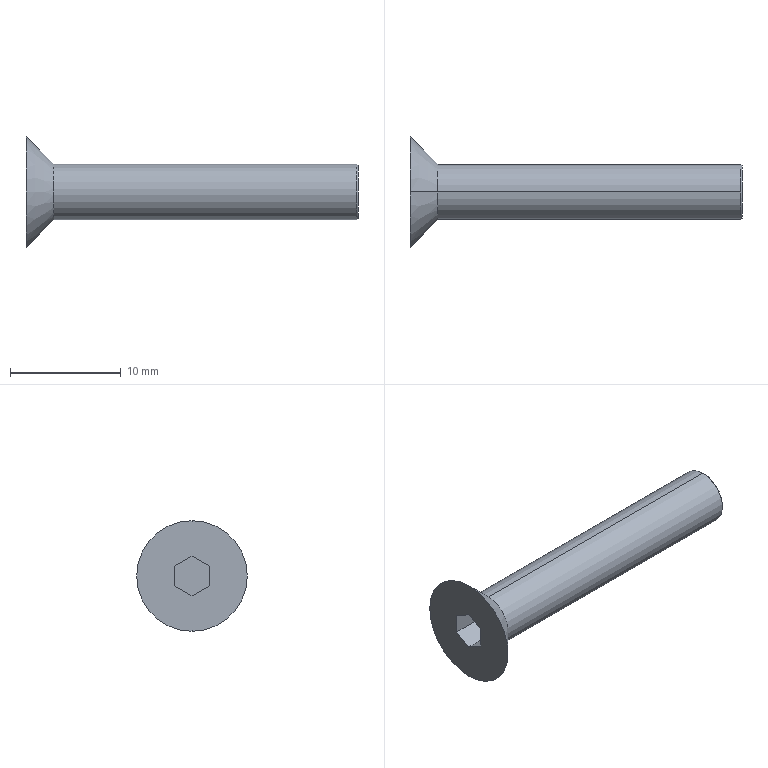Part | SolidWorks | features BaseBody 1 | 1 solid | 15 faces | box 30 x 10 x 10 mm | volume 635.279 mm3 | plane 9 | cone 4 | cylinder 2 | commonest cylinder face diameters 5 x2
STEP:
#1=CARTESIAN_POINT('',(29.9,0.,2.5));
#2=VERTEX_POINT('',#1);
#3=CARTESIAN_POINT('',(29.9,0.,-2.5));
#4=VERTEX_POINT('',#3);
#5=CARTESIAN_POINT('',(29.9,0.,0.));
#6=DIRECTION('',(-1.,0.,0.));
#7=DIRECTION('',(0.,0.,1.));
#8=AXIS2_PLACEMENT_3D('',#5,#6,#7);
#9=CIRCLE('',#8,2.5);
#10=EDGE_CURVE('',#2,#4,#9,.T.);
#11=ORIENTED_EDGE('',*,*,#10,.T.);
#12=CARTESIAN_POINT('',(2.5,0.,-2.5));
#13=VERTEX_POINT('',#12);
#14=CARTESIAN_POINT('',(0.,0.,-2.5));
#15=DIRECTION('',(-1.,0.,0.));
#16=VECTOR('',#15,1000.);
#17=LINE('',#14,#16);
#18=EDGE_CURVE('',#4,#13,#17,.T.);
#19=ORIENTED_EDGE('',*,*,#18,.T.);
#20=CARTESIAN_POINT('',(2.5,0.,2.5));
#21=VERTEX_POINT('',#20);
#22=CARTESIAN_POINT('',(2.5,0.,0.));
#23=DIRECTION('',(1.,0.,0.));
#24=DIRECTION('',(0.,0.,1.));
#25=AXIS2_PLACEMENT_3D('',#22,#23,#24);
#26=CIRCLE('',#25,2.5);
#27=EDGE_CURVE('',#13,#21,#26,.T.);
#28=ORIENTED_EDGE('',*,*,#27,.T.);
#29=CARTESIAN_POINT('',(0.,0.,2.5));
#30=DIRECTION('',(-1.,0.,0.));
#31=VECTOR('',#30,1000.);
#32=LINE('',#29,#31);
#33=EDGE_CURVE('',#2,#21,#32,.T.);
#34=ORIENTED_EDGE('',*,*,#33,.F.);
#35=EDGE_LOOP('',(#11,#19,#28,#34));
#36=FACE_OUTER_BOUND('',#35,.T.);
#37=CARTESIAN_POINT('',(0.,0.,0.));
#38=DIRECTION('',(-1.,0.,0.));
#39=DIRECTION('',(0.,0.,1.));
#40=AXIS2_PLACEMENT_3D('',#37,#38,#39);
#41=CYLINDRICAL_SURFACE('',#40,2.5);
#42=ADVANCED_FACE('',(#36),#41,.T.);
#43=ORIENTED_EDGE('',*,*,#27,.F.);
#44=CARTESIAN_POINT('',(0.,0.,-5.));
#45=VERTEX_POINT('',#44);
#46=CARTESIAN_POINT('',(0.,0.,-5.));
#47=DIRECTION('',(-0.7071,0.,-0.7071));
#48=VECTOR('',#47,1000.);
#49=LINE('',#46,#48);
#50=EDGE_CURVE('',#13,#45,#49,.T.);
#51=ORIENTED_EDGE('',*,*,#50,.T.);
#52=CARTESIAN_POINT('',(0.,0.,5.));
#53=VERTEX_POINT('',#52);
#54=CARTESIAN_POINT('',(0.,0.,0.));
#55=DIRECTION('',(1.,0.,0.));
#56=DIRECTION('',(0.,0.,1.));
#57=AXIS2_PLACEMENT_3D('',#54,#55,#56);
#58=CIRCLE('',#57,5.);
#59=EDGE_CURVE('',#45,#53,#58,.T.);
#60=ORIENTED_EDGE('',*,*,#59,.T.);
#61=CARTESIAN_POINT('',(0.,0.,5.));
#62=DIRECTION('',(-0.7071,0.,0.7071));
#63=VECTOR('',#62,1000.);
#64=LINE('',#61,#63);
#65=EDGE_CURVE('',#21,#53,#64,.T.);
#66=ORIENTED_EDGE('',*,*,#65,.F.);
#67=EDGE_LOOP('',(#43,#51,#60,#66));
#68=FACE_OUTER_BOUND('',#67,.T.);
#69=CARTESIAN_POINT('',(0.,0.,0.));
#70=DIRECTION('',(-1.,0.,0.));
#71=DIRECTION('',(0.,0.,1.));
#72=AXIS2_PLACEMENT_3D('',#69,#70,#71);
#73=CONICAL_SURFACE('',#72,5.,0.7854);
#74=ADVANCED_FACE('',(#68),#73,.T.);
#75=CARTESIAN_POINT('',(30.,0.,2.4));
#76=VERTEX_POINT('',#75);
#77=CARTESIAN_POINT('',(30.,0.,-2.4));
#78=VERTEX_POINT('',#77);
#79=CARTESIAN_POINT('',(30.,0.,0.));
#80=DIRECTION('',(-1.,0.,0.));
#81=DIRECTION('',(0.,0.,1.));
#82=AXIS2_PLACEMENT_3D('',#79,#80,#81);
#83=CIRCLE('',#82,2.4);
#84=EDGE_CURVE('',#76,#78,#83,.T.);
#85=ORIENTED_EDGE('',*,*,#84,.T.);
#86=CARTESIAN_POINT('',(29.9,0.,-2.5));
#87=DIRECTION('',(-0.7071,0.,-0.7071));
#88=VECTOR('',#87,1000.);
#89=LINE('',#86,#88);
#90=EDGE_CURVE('',#78,#4,#89,.T.);
#91=ORIENTED_EDGE('',*,*,#90,.T.);
#92=ORIENTED_EDGE('',*,*,#10,.F.);
#93=CARTESIAN_POINT('',(29.9,0.,2.5));
#94=DIRECTION('',(-0.7071,0.,0.7071));
#95=VECTOR('',#94,1000.);
#96=LINE('',#93,#95);
#97=EDGE_CURVE('',#76,#2,#96,.T.);
#98=ORIENTED_EDGE('',*,*,#97,.F.);
#99=EDGE_LOOP('',(#85,#91,#92,#98));
#100=FACE_OUTER_BOUND('',#99,.T.);
#101=CARTESIAN_POINT('',(29.9,0.,0.));
#102=DIRECTION('',(-1.,0.,0.));
#103=DIRECTION('',(0.,0.,1.));
#104=AXIS2_PLACEMENT_3D('',#101,#102,#103);
#105=CONICAL_SURFACE('',#104,2.5,0.7854);
#106=ADVANCED_FACE('',(#100),#105,.T.);
#107=ORIENTED_EDGE('',*,*,#18,.F.);
#108=CARTESIAN_POINT('',(29.9,0.,0.));
#109=DIRECTION('',(-1.,0.,0.));
#110=DIRECTION('',(0.,0.,1.));
#111=AXIS2_PLACEMENT_3D('',#108,#109,#110);
#112=CIRCLE('',#111,2.5);
#113=EDGE_CURVE('',#4,#2,#112,.T.);
#114=ORIENTED_EDGE('',*,*,#113,.T.);
#115=ORIENTED_EDGE('',*,*,#33,.T.);
#116=CARTESIAN_POINT('',(2.5,0.,0.));
#117=DIRECTION('',(1.,0.,0.));
#118=DIRECTION('',(0.,0.,1.));
#119=AXIS2_PLACEMENT_3D('',#116,#117,#118);
#120=CIRCLE('',#119,2.5);
#121=EDGE_CURVE('',#21,#13,#120,.T.);
#122=ORIENTED_EDGE('',*,*,#121,.T.);
#123=EDGE_LOOP('',(#107,#114,#115,#122));
#124=FACE_OUTER_BOUND('',#123,.T.);
#125=CARTESIAN_POINT('',(0.,0.,0.));
#126=DIRECTION('',(-1.,0.,0.));
#127=DIRECTION('',(0.,0.,1.));
#128=AXIS2_PLACEMENT_3D('',#125,#126,#127);
#129=CYLINDRICAL_SURFACE('',#128,2.5);
#130=ADVANCED_FACE('',(#124),#129,.T.);
#131=ORIENTED_EDGE('',*,*,#50,.F.);
#132=ORIENTED_EDGE('',*,*,#121,.F.);
#133=ORIENTED_EDGE('',*,*,#65,.T.);
#134=CARTESIAN_POINT('',(0.,0.,0.));
#135=DIRECTION('',(1.,0.,0.));
#136=DIRECTION('',(0.,0.,1.));
#137=AXIS2_PLACEMENT_3D('',#134,#135,#136);
#138=CIRCLE('',#137,5.);
#139=EDGE_CURVE('',#53,#45,#138,.T.);
#140=ORIENTED_EDGE('',*,*,#139,.T.);
#141=EDGE_LOOP('',(#131,#132,#133,#140));
#142=FACE_OUTER_BOUND('',#141,.T.);
#143=CARTESIAN_POINT('',(0.,0.,0.));
#144=DIRECTION('',(-1.,0.,0.));
#145=DIRECTION('',(0.,0.,1.));
#146=AXIS2_PLACEMENT_3D('',#143,#144,#145);
#147=CONICAL_SURFACE('',#146,5.,0.7854);
#148=ADVANCED_FACE('',(#142),#147,.T.);
#149=ORIENTED_EDGE('',*,*,#90,.F.);
#150=CARTESIAN_POINT('',(30.,0.,0.));
#151=DIRECTION('',(-1.,0.,0.));
#152=DIRECTION('',(0.,0.,1.));
#153=AXIS2_PLACEMENT_3D('',#150,#151,#152);
#154=CIRCLE('',#153,2.4);
#155=EDGE_CURVE('',#78,#76,#154,.T.);
#156=ORIENTED_EDGE('',*,*,#155,.T.);
#157=ORIENTED_EDGE('',*,*,#97,.T.);
#158=ORIENTED_EDGE('',*,*,#113,.F.);
#159=EDGE_LOOP('',(#149,#156,#157,#158));
#160=FACE_OUTER_BOUND('',#159,.T.);
#161=CARTESIAN_POINT('',(29.9,0.,0.));
#162=DIRECTION('',(-1.,0.,0.));
#163=DIRECTION('',(0.,0.,1.));
#164=AXIS2_PLACEMENT_3D('',#161,#162,#163);
#165=CONICAL_SURFACE('',#164,2.5,0.7854);
#166=ADVANCED_FACE('',(#160),#165,.T.);
#167=ORIENTED_EDGE('',*,*,#139,.F.);
#168=ORIENTED_EDGE('',*,*,#59,.F.);
#169=EDGE_LOOP('',(#167,#168));
#170=FACE_OUTER_BOUND('',#169,.T.);
#171=CARTESIAN_POINT('',(0.,-1.55,0.8949));
#172=VERTEX_POINT('',#171);
#173=CARTESIAN_POINT('',(0.,0.,1.79));
#174=VERTEX_POINT('',#173);
#175=CARTESIAN_POINT('',(0.,-1.55,0.8949));
#176=DIRECTION('',(0.,0.866,0.5));
#177=VECTOR('',#176,1000.);
#178=LINE('',#175,#177);
#179=EDGE_CURVE('',#172,#174,#178,.T.);
#180=ORIENTED_EDGE('',*,*,#179,.F.);
#181=CARTESIAN_POINT('',(0.,-1.55,-0.8949));
#182=VERTEX_POINT('',#181);
#183=CARTESIAN_POINT('',(0.,-1.55,0.));
#184=DIRECTION('',(0.,0.,1.));
#185=VECTOR('',#184,1000.);
#186=LINE('',#183,#185);
#187=EDGE_CURVE('',#182,#172,#186,.T.);
#188=ORIENTED_EDGE('',*,*,#187,.F.);
#189=CARTESIAN_POINT('',(0.,0.,-1.79));
#190=VERTEX_POINT('',#189);
#191=CARTESIAN_POINT('',(0.,0.,-1.79));
#192=DIRECTION('',(0.,-0.866,0.5));
#193=VECTOR('',#192,1000.);
#194=LINE('',#191,#193);
#195=EDGE_CURVE('',#190,#182,#194,.T.);
#196=ORIENTED_EDGE('',*,*,#195,.F.);
#197=CARTESIAN_POINT('',(0.,1.55,-0.8949));
#198=VERTEX_POINT('',#197);
#199=CARTESIAN_POINT('',(0.,1.55,-0.8949));
#200=DIRECTION('',(0.,-0.866,-0.5));
#201=VECTOR('',#200,1000.);
#202=LINE('',#199,#201);
#203=EDGE_CURVE('',#198,#190,#202,.T.);
#204=ORIENTED_EDGE('',*,*,#203,.F.);
#205=CARTESIAN_POINT('',(0.,1.55,0.8949));
#206=VERTEX_POINT('',#205);
#207=CARTESIAN_POINT('',(0.,1.55,0.));
#208=DIRECTION('',(0.,0.,-1.));
#209=VECTOR('',#208,1000.);
#210=LINE('',#207,#209);
#211=EDGE_CURVE('',#206,#198,#210,.T.);
#212=ORIENTED_EDGE('',*,*,#211,.F.);
#213=CARTESIAN_POINT('',(0.,0.,1.79));
#214=DIRECTION('',(0.,0.866,-0.5));
#215=VECTOR('',#214,1000.);
#216=LINE('',#213,#215);
#217=EDGE_CURVE('',#174,#206,#216,.T.);
#218=ORIENTED_EDGE('',*,*,#217,.F.);
#219=EDGE_LOOP('',(#180,#188,#196,#204,#212,#218));
#220=FACE_BOUND('',#219,.T.);
#221=CARTESIAN_POINT('',(0.,0.,0.));
#222=DIRECTION('',(1.,0.,0.));
#223=DIRECTION('',(0.,0.,-1.));
#224=AXIS2_PLACEMENT_3D('',#221,#222,#223);
#225=PLANE('',#224);
#226=ADVANCED_FACE('',(#170,#220),#225,.F.);
#227=ORIENTED_EDGE('',*,*,#84,.F.);
#228=ORIENTED_EDGE('',*,*,#155,.F.);
#229=EDGE_LOOP('',(#227,#228));
#230=FACE_OUTER_BOUND('',#229,.T.);
#231=CARTESIAN_POINT('',(30.,0.,-2.5));
#232=DIRECTION('',(-1.,0.,0.));
#233=DIRECTION('',(0.,0.,1.));
#234=AXIS2_PLACEMENT_3D('',#231,#232,#233);
#235=PLANE('',#234);
#236=ADVANCED_FACE('',(#230),#235,.F.);
#237=CARTESIAN_POINT('',(2.3,1.55,0.8949));
#238=VERTEX_POINT('',#237);
#239=CARTESIAN_POINT('',(2.3,1.55,0.8949));
#240=DIRECTION('',(-1.,0.,0.));
#241=VECTOR('',#240,1000.);
#242=LINE('',#239,#241);
#243=EDGE_CURVE('',#238,#206,#242,.T.);
#244=ORIENTED_EDGE('',*,*,#243,.F.);
#245=CARTESIAN_POINT('',(2.3,0.,1.79));
#246=VERTEX_POINT('',#245);
#247=CARTESIAN_POINT('',(2.3,0.,1.79));
#248=DIRECTION('',(0.,0.866,-0.5));
#249=VECTOR('',#248,1000.);
#250=LINE('',#247,#249);
#251=EDGE_CURVE('',#246,#238,#250,.T.);
#252=ORIENTED_EDGE('',*,*,#251,.F.);
#253=CARTESIAN_POINT('',(2.3,0.,1.79));
#254=DIRECTION('',(1.,0.,0.));
#255=VECTOR('',#254,1000.);
#256=LINE('',#253,#255);
#257=EDGE_CURVE('',#174,#246,#256,.T.);
#258=ORIENTED_EDGE('',*,*,#257,.F.);
#259=ORIENTED_EDGE('',*,*,#217,.T.);
#260=EDGE_LOOP('',(#244,#252,#258,#259));
#261=FACE_OUTER_BOUND('',#260,.T.);
#262=CARTESIAN_POINT('',(2.3,0.,1.79));
#263=DIRECTION('',(0.,0.5,0.866));
#264=DIRECTION('',(0.,-0.866,0.5));
#265=AXIS2_PLACEMENT_3D('',#262,#263,#264);
#266=PLANE('',#265);
#267=ADVANCED_FACE('',(#261),#266,.F.);
#268=ORIENTED_EDGE('',*,*,#257,.T.);
#269=CARTESIAN_POINT('',(2.3,-1.55,0.8949));
#270=VERTEX_POINT('',#269);
#271=CARTESIAN_POINT('',(2.3,-1.55,0.8949));
#272=DIRECTION('',(0.,0.866,0.5));
#273=VECTOR('',#272,1000.);
#274=LINE('',#271,#273);
#275=EDGE_CURVE('',#270,#246,#274,.T.);
#276=ORIENTED_EDGE('',*,*,#275,.F.);
#277=CARTESIAN_POINT('',(2.3,-1.55,0.8949));
#278=DIRECTION('',(1.,0.,0.));
#279=VECTOR('',#278,1000.);
#280=LINE('',#277,#279);
#281=EDGE_CURVE('',#172,#270,#280,.T.);
#282=ORIENTED_EDGE('',*,*,#281,.F.);
#283=ORIENTED_EDGE('',*,*,#179,.T.);
#284=EDGE_LOOP('',(#268,#276,#282,#283));
#285=FACE_OUTER_BOUND('',#284,.T.);
#286=CARTESIAN_POINT('',(2.3,-1.55,0.8949));
#287=DIRECTION('',(0.,-0.5,0.866));
#288=DIRECTION('',(0.,-0.866,-0.5));
#289=AXIS2_PLACEMENT_3D('',#286,#287,#288);
#290=PLANE('',#289);
#291=ADVANCED_FACE('',(#285),#290,.F.);
#292=ORIENTED_EDGE('',*,*,#281,.T.);
#293=CARTESIAN_POINT('',(2.3,-1.55,-0.8949));
#294=VERTEX_POINT('',#293);
#295=CARTESIAN_POINT('',(2.3,-1.55,-0.8949));
#296=DIRECTION('',(0.,0.,1.));
#297=VECTOR('',#296,1000.);
#298=LINE('',#295,#297);
#299=EDGE_CURVE('',#294,#270,#298,.T.);
#300=ORIENTED_EDGE('',*,*,#299,.F.);
#301=CARTESIAN_POINT('',(2.3,-1.55,-0.8949));
#302=DIRECTION('',(1.,0.,0.));
#303=VECTOR('',#302,1000.);
#304=LINE('',#301,#303);
#305=EDGE_CURVE('',#182,#294,#304,.T.);
#306=ORIENTED_EDGE('',*,*,#305,.F.);
#307=ORIENTED_EDGE('',*,*,#187,.T.);
#308=EDGE_LOOP('',(#292,#300,#306,#307));
#309=FACE_OUTER_BOUND('',#308,.T.);
#310=CARTESIAN_POINT('',(2.3,-1.55,-0.8949));
#311=DIRECTION('',(0.,-1.,0.));
#312=DIRECTION('',(0.,0.,-1.));
#313=AXIS2_PLACEMENT_3D('',#310,#311,#312);
#314=PLANE('',#313);
#315=ADVANCED_FACE('',(#309),#314,.F.);
#316=ORIENTED_EDGE('',*,*,#305,.T.);
#317=CARTESIAN_POINT('',(2.3,0.,-1.79));
#318=VERTEX_POINT('',#317);
#319=CARTESIAN_POINT('',(2.3,0.,-1.79));
#320=DIRECTION('',(0.,-0.866,0.5));
#321=VECTOR('',#320,1000.);
#322=LINE('',#319,#321);
#323=EDGE_CURVE('',#318,#294,#322,.T.);
#324=ORIENTED_EDGE('',*,*,#323,.F.);
#325=CARTESIAN_POINT('',(2.3,0.,-1.79));
#326=DIRECTION('',(1.,0.,0.));
#327=VECTOR('',#326,1000.);
#328=LINE('',#325,#327);
#329=EDGE_CURVE('',#190,#318,#328,.T.);
#330=ORIENTED_EDGE('',*,*,#329,.F.);
#331=ORIENTED_EDGE('',*,*,#195,.T.);
#332=EDGE_LOOP('',(#316,#324,#330,#331));
#333=FACE_OUTER_BOUND('',#332,.T.);
#334=CARTESIAN_POINT('',(2.3,0.,-1.79));
#335=DIRECTION('',(0.,-0.5,-0.866));
#336=DIRECTION('',(0.,0.866,-0.5));
#337=AXIS2_PLACEMENT_3D('',#334,#335,#336);
#338=PLANE('',#337);
#339=ADVANCED_FACE('',(#333),#338,.F.);
#340=ORIENTED_EDGE('',*,*,#329,.T.);
#341=CARTESIAN_POINT('',(2.3,1.55,-0.8949));
#342=VERTEX_POINT('',#341);
#343=CARTESIAN_POINT('',(2.3,1.55,-0.8949));
#344=DIRECTION('',(0.,-0.866,-0.5));
#345=VECTOR('',#344,1000.);
#346=LINE('',#343,#345);
#347=EDGE_CURVE('',#342,#318,#346,.T.);
#348=ORIENTED_EDGE('',*,*,#347,.F.);
#349=CARTESIAN_POINT('',(2.3,1.55,-0.8949));
#350=DIRECTION('',(1.,0.,0.));
#351=VECTOR('',#350,1000.);
#352=LINE('',#349,#351);
#353=EDGE_CURVE('',#198,#342,#352,.T.);
#354=ORIENTED_EDGE('',*,*,#353,.F.);
#355=ORIENTED_EDGE('',*,*,#203,.T.);
#356=EDGE_LOOP('',(#340,#348,#354,#355));
#357=FACE_OUTER_BOUND('',#356,.T.);
#358=CARTESIAN_POINT('',(2.3,1.55,-0.8949));
#359=DIRECTION('',(0.,0.5,-0.866));
#360=DIRECTION('',(0.,0.866,0.5));
#361=AXIS2_PLACEMENT_3D('',#358,#359,#360);
#362=PLANE('',#361);
#363=ADVANCED_FACE('',(#357),#362,.F.);
#364=ORIENTED_EDGE('',*,*,#353,.T.);
#365=CARTESIAN_POINT('',(2.3,1.55,0.8949));
#366=DIRECTION('',(0.,0.,-1.));
#367=VECTOR('',#366,1000.);
#368=LINE('',#365,#367);
#369=EDGE_CURVE('',#238,#342,#368,.T.);
#370=ORIENTED_EDGE('',*,*,#369,.F.);
#371=ORIENTED_EDGE('',*,*,#243,.T.);
#372=ORIENTED_EDGE('',*,*,#211,.T.);
#373=EDGE_LOOP('',(#364,#370,#371,#372));
#374=FACE_OUTER_BOUND('',#373,.T.);
#375=CARTESIAN_POINT('',(2.3,1.55,0.8949));
#376=DIRECTION('',(0.,1.,0.));
#377=DIRECTION('',(0.,0.,1.));
#378=AXIS2_PLACEMENT_3D('',#375,#376,#377);
#379=PLANE('',#378);
#380=ADVANCED_FACE('',(#374),#379,.F.);
#381=ORIENTED_EDGE('',*,*,#323,.T.);
#382=ORIENTED_EDGE('',*,*,#299,.T.);
#383=ORIENTED_EDGE('',*,*,#275,.T.);
#384=ORIENTED_EDGE('',*,*,#251,.T.);
#385=ORIENTED_EDGE('',*,*,#369,.T.);
#386=ORIENTED_EDGE('',*,*,#347,.T.);
#387=EDGE_LOOP('',(#381,#382,#383,#384,#385,#386));
#388=FACE_OUTER_BOUND('',#387,.T.);
#389=CARTESIAN_POINT('',(2.3,0.,0.));
#390=DIRECTION('',(-1.,0.,0.));
#391=DIRECTION('',(0.,0.,1.));
#392=AXIS2_PLACEMENT_3D('',#389,#390,#391);
#393=PLANE('',#392);
#394=ADVANCED_FACE('',(#388),#393,.T.);
#395=CLOSED_SHELL('',(#42,#74,#106,#130,#148,#166,#226,#236,#267,#291,#315,#339,#363,#380,#394));
#396=MANIFOLD_SOLID_BREP('',#395);
#397=CARTESIAN_POINT('',(0.,0.,0.));
#398=DIRECTION('',(0.,0.,1.));
#399=DIRECTION('',(1.,0.,0.));
#400=AXIS2_PLACEMENT_3D('',#397,#398,#399);
#401=(LENGTH_UNIT()NAMED_UNIT(*)SI_UNIT(.MILLI.,.METRE.));
#402=UNCERTAINTY_MEASURE_WITH_UNIT(LENGTH_MEASURE(0.00001),#401,'','');
#403=(NAMED_UNIT(*)PLANE_ANGLE_UNIT()SI_UNIT($,.RADIAN.));
#404=(NAMED_UNIT(*)SI_UNIT($,.STERADIAN.)SOLID_ANGLE_UNIT());
#405=(GEOMETRIC_REPRESENTATION_CONTEXT(3)GLOBAL_UNCERTAINTY_ASSIGNED_CONTEXT((#402))GLOBAL_UNIT_ASSIGNED_CONTEXT((#401,#403,#404))REPRESENTATION_CONTEXT('',''));
#406=ADVANCED_BREP_SHAPE_REPRESENTATION('',(#396,#400),#405);